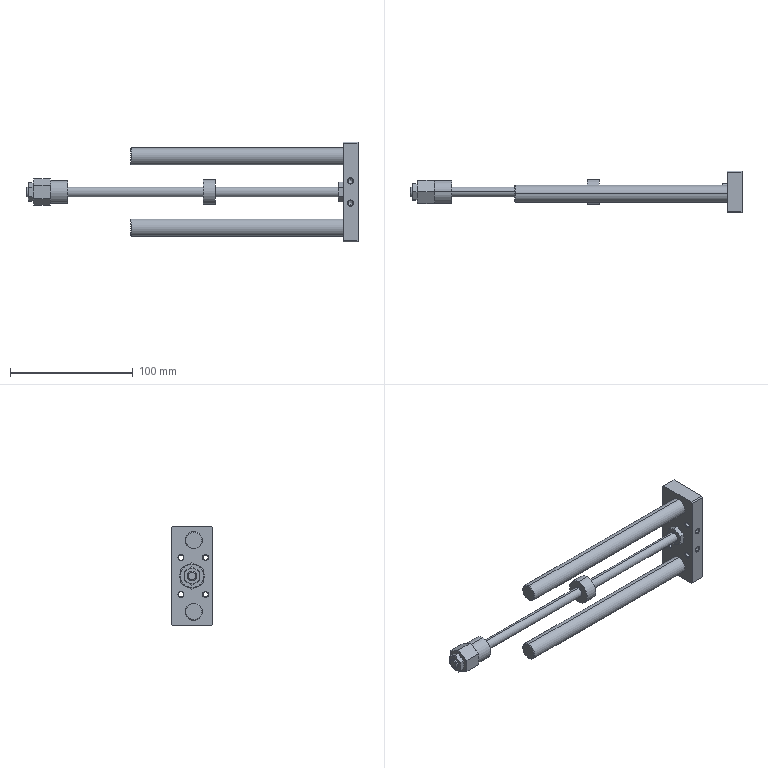Part | SolidWorks | features RefAxis 9, RevCut 7, Revolution 6, ICE 4, 3DProfileFeature 3, HoleWzd 2, Extrusion 1 | 1 solid | 174 faces | box 270 x 34 x 81 mm | volume 107228 mm3 | cone 84 | plane 50 | cylinder 40 | commonest cylinder face diameters 4.134 x16 9 x8 8 x6 14 x4 18.62 x2 20 x2